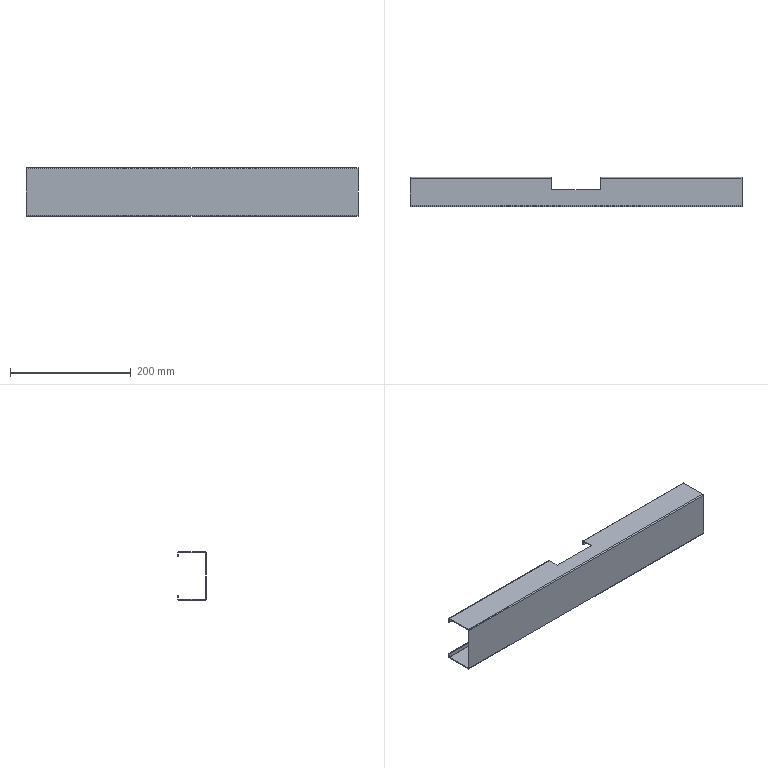Part | 1 solid | 62 faces | box 550 x 48 x 80 mm | volume 145842 mm3 | plane 50 | cylinder 12 | commonest cylinder face diameters 0.4 x6 3.4 x6
STEP:
#1=CARTESIAN_POINT('',(-40.,48.,38.3));
#2=VERTEX_POINT('',#1);
#3=CARTESIAN_POINT('',(-40.,48.,32.));
#4=VERTEX_POINT('',#3);
#5=CARTESIAN_POINT('',(-40.,48.,32.));
#6=DIRECTION('',(0.,0.,-1.));
#7=VECTOR('',#6,1000.);
#8=LINE('',#5,#7);
#9=EDGE_CURVE('',#2,#4,#8,.T.);
#10=ORIENTED_EDGE('',*,*,#9,.F.);
#11=CARTESIAN_POINT('',(-40.,46.5,38.3));
#12=VERTEX_POINT('',#11);
#13=CARTESIAN_POINT('',(-40.,48.,38.3));
#14=DIRECTION('',(0.,-1.,0.));
#15=VECTOR('',#14,1000.);
#16=LINE('',#13,#15);
#17=EDGE_CURVE('',#2,#12,#16,.T.);
#18=ORIENTED_EDGE('',*,*,#17,.T.);
#19=CARTESIAN_POINT('',(-40.,46.5,32.));
#20=VERTEX_POINT('',#19);
#21=CARTESIAN_POINT('',(-40.,46.5,32.));
#22=DIRECTION('',(0.,0.,-1.));
#23=VECTOR('',#22,1000.);
#24=LINE('',#21,#23);
#25=EDGE_CURVE('',#12,#20,#24,.T.);
#26=ORIENTED_EDGE('',*,*,#25,.T.);
#27=CARTESIAN_POINT('',(-40.,48.,32.));
#28=DIRECTION('',(0.,1.,0.));
#29=VECTOR('',#28,1000.);
#30=LINE('',#27,#29);
#31=EDGE_CURVE('',#20,#4,#30,.T.);
#32=ORIENTED_EDGE('',*,*,#31,.T.);
#33=EDGE_LOOP('',(#10,#18,#26,#32));
#34=FACE_OUTER_BOUND('',#33,.T.);
#35=CARTESIAN_POINT('',(-40.,68.,-40.));
#36=DIRECTION('',(-1.,0.,0.));
#37=DIRECTION('',(0.,0.,1.));
#38=AXIS2_PLACEMENT_3D('',#35,#36,#37);
#39=PLANE('',#38);
#40=ADVANCED_FACE('',(#34),#39,.F.);
#41=CARTESIAN_POINT('',(-40.,28.,38.5));
#42=VERTEX_POINT('',#41);
#43=CARTESIAN_POINT('',(-40.,46.3,38.5));
#44=VERTEX_POINT('',#43);
#45=CARTESIAN_POINT('',(-40.,48.,38.5));
#46=DIRECTION('',(0.,1.,0.));
#47=VECTOR('',#46,1000.);
#48=LINE('',#45,#47);
#49=EDGE_CURVE('',#42,#44,#48,.T.);
#50=ORIENTED_EDGE('',*,*,#49,.T.);
#51=CARTESIAN_POINT('',(-40.,46.3,40.));
#52=VERTEX_POINT('',#51);
#53=CARTESIAN_POINT('',(-40.,46.3,38.5));
#54=DIRECTION('',(0.,0.,1.));
#55=VECTOR('',#54,1000.);
#56=LINE('',#53,#55);
#57=EDGE_CURVE('',#44,#52,#56,.T.);
#58=ORIENTED_EDGE('',*,*,#57,.T.);
#59=CARTESIAN_POINT('',(-40.,28.,40.));
#60=VERTEX_POINT('',#59);
#61=CARTESIAN_POINT('',(-40.,48.,40.));
#62=DIRECTION('',(0.,1.,0.));
#63=VECTOR('',#62,1000.);
#64=LINE('',#61,#63);
#65=EDGE_CURVE('',#60,#52,#64,.T.);
#66=ORIENTED_EDGE('',*,*,#65,.F.);
#67=CARTESIAN_POINT('',(-40.,28.,-40.));
#68=DIRECTION('',(0.,0.,1.));
#69=VECTOR('',#68,1000.);
#70=LINE('',#67,#69);
#71=EDGE_CURVE('',#42,#60,#70,.T.);
#72=ORIENTED_EDGE('',*,*,#71,.F.);
#73=EDGE_LOOP('',(#50,#58,#66,#72));
#74=FACE_OUTER_BOUND('',#73,.T.);
#75=CARTESIAN_POINT('',(-40.,68.,-40.));
#76=DIRECTION('',(-1.,0.,0.));
#77=DIRECTION('',(0.,0.,1.));
#78=AXIS2_PLACEMENT_3D('',#75,#76,#77);
#79=PLANE('',#78);
#80=ADVANCED_FACE('',(#74),#79,.F.);
#81=CARTESIAN_POINT('',(40.,46.5,32.));
#82=VERTEX_POINT('',#81);
#83=CARTESIAN_POINT('',(40.,46.5,38.3));
#84=VERTEX_POINT('',#83);
#85=CARTESIAN_POINT('',(40.,46.5,32.));
#86=DIRECTION('',(0.,0.,1.));
#87=VECTOR('',#86,1000.);
#88=LINE('',#85,#87);
#89=EDGE_CURVE('',#82,#84,#88,.T.);
#90=ORIENTED_EDGE('',*,*,#89,.T.);
#91=CARTESIAN_POINT('',(40.,48.,38.3));
#92=VERTEX_POINT('',#91);
#93=CARTESIAN_POINT('',(40.,46.5,38.3));
#94=DIRECTION('',(0.,1.,0.));
#95=VECTOR('',#94,1000.);
#96=LINE('',#93,#95);
#97=EDGE_CURVE('',#84,#92,#96,.T.);
#98=ORIENTED_EDGE('',*,*,#97,.T.);
#99=CARTESIAN_POINT('',(40.,48.,32.));
#100=VERTEX_POINT('',#99);
#101=CARTESIAN_POINT('',(40.,48.,32.));
#102=DIRECTION('',(0.,0.,1.));
#103=VECTOR('',#102,1000.);
#104=LINE('',#101,#103);
#105=EDGE_CURVE('',#100,#92,#104,.T.);
#106=ORIENTED_EDGE('',*,*,#105,.F.);
#107=CARTESIAN_POINT('',(40.,48.,32.));
#108=DIRECTION('',(0.,-1.,0.));
#109=VECTOR('',#108,1000.);
#110=LINE('',#107,#109);
#111=EDGE_CURVE('',#100,#82,#110,.T.);
#112=ORIENTED_EDGE('',*,*,#111,.T.);
#113=EDGE_LOOP('',(#90,#98,#106,#112));
#114=FACE_OUTER_BOUND('',#113,.T.);
#115=CARTESIAN_POINT('',(40.,68.,-40.));
#116=DIRECTION('',(1.,0.,0.));
#117=DIRECTION('',(0.,1.,0.));
#118=AXIS2_PLACEMENT_3D('',#115,#116,#117);
#119=PLANE('',#118);
#120=ADVANCED_FACE('',(#114),#119,.F.);
#121=CARTESIAN_POINT('',(40.,46.3,40.));
#122=VERTEX_POINT('',#121);
#123=CARTESIAN_POINT('',(40.,28.,40.));
#124=VERTEX_POINT('',#123);
#125=CARTESIAN_POINT('',(40.,48.,40.));
#126=DIRECTION('',(0.,-1.,0.));
#127=VECTOR('',#126,1000.);
#128=LINE('',#125,#127);
#129=EDGE_CURVE('',#122,#124,#128,.T.);
#130=ORIENTED_EDGE('',*,*,#129,.F.);
#131=CARTESIAN_POINT('',(40.,46.3,38.5));
#132=VERTEX_POINT('',#131);
#133=CARTESIAN_POINT('',(40.,46.3,40.));
#134=DIRECTION('',(0.,0.,-1.));
#135=VECTOR('',#134,1000.);
#136=LINE('',#133,#135);
#137=EDGE_CURVE('',#122,#132,#136,.T.);
#138=ORIENTED_EDGE('',*,*,#137,.T.);
#139=CARTESIAN_POINT('',(40.,28.,38.5));
#140=VERTEX_POINT('',#139);
#141=CARTESIAN_POINT('',(40.,48.,38.5));
#142=DIRECTION('',(0.,-1.,0.));
#143=VECTOR('',#142,1000.);
#144=LINE('',#141,#143);
#145=EDGE_CURVE('',#132,#140,#144,.T.);
#146=ORIENTED_EDGE('',*,*,#145,.T.);
#147=CARTESIAN_POINT('',(40.,28.,-40.));
#148=DIRECTION('',(0.,0.,1.));
#149=VECTOR('',#148,1000.);
#150=LINE('',#147,#149);
#151=EDGE_CURVE('',#140,#124,#150,.T.);
#152=ORIENTED_EDGE('',*,*,#151,.T.);
#153=EDGE_LOOP('',(#130,#138,#146,#152));
#154=FACE_OUTER_BOUND('',#153,.T.);
#155=CARTESIAN_POINT('',(40.,68.,-40.));
#156=DIRECTION('',(1.,0.,0.));
#157=DIRECTION('',(0.,1.,0.));
#158=AXIS2_PLACEMENT_3D('',#155,#156,#157);
#159=PLANE('',#158);
#160=ADVANCED_FACE('',(#154),#159,.F.);
#161=CARTESIAN_POINT('',(-40.,46.5,-32.));
#162=VERTEX_POINT('',#161);
#163=CARTESIAN_POINT('',(-40.,46.5,-38.3));
#164=VERTEX_POINT('',#163);
#165=CARTESIAN_POINT('',(-40.,46.5,-40.));
#166=DIRECTION('',(0.,0.,-1.));
#167=VECTOR('',#166,1000.);
#168=LINE('',#165,#167);
#169=EDGE_CURVE('',#162,#164,#168,.T.);
#170=ORIENTED_EDGE('',*,*,#169,.T.);
#171=CARTESIAN_POINT('',(-40.,48.,-38.3));
#172=VERTEX_POINT('',#171);
#173=CARTESIAN_POINT('',(-40.,46.5,-38.3));
#174=DIRECTION('',(0.,1.,0.));
#175=VECTOR('',#174,1000.);
#176=LINE('',#173,#175);
#177=EDGE_CURVE('',#164,#172,#176,.T.);
#178=ORIENTED_EDGE('',*,*,#177,.T.);
#179=CARTESIAN_POINT('',(-40.,48.,-32.));
#180=VERTEX_POINT('',#179);
#181=CARTESIAN_POINT('',(-40.,48.,-40.));
#182=DIRECTION('',(0.,0.,-1.));
#183=VECTOR('',#182,1000.);
#184=LINE('',#181,#183);
#185=EDGE_CURVE('',#180,#172,#184,.T.);
#186=ORIENTED_EDGE('',*,*,#185,.F.);
#187=CARTESIAN_POINT('',(-40.,46.5,-32.));
#188=DIRECTION('',(0.,-1.,0.));
#189=VECTOR('',#188,1000.);
#190=LINE('',#187,#189);
#191=EDGE_CURVE('',#180,#162,#190,.T.);
#192=ORIENTED_EDGE('',*,*,#191,.T.);
#193=EDGE_LOOP('',(#170,#178,#186,#192));
#194=FACE_OUTER_BOUND('',#193,.T.);
#195=CARTESIAN_POINT('',(-40.,68.,-40.));
#196=DIRECTION('',(-1.,0.,0.));
#197=DIRECTION('',(0.,0.,1.));
#198=AXIS2_PLACEMENT_3D('',#195,#196,#197);
#199=PLANE('',#198);
#200=ADVANCED_FACE('',(#194),#199,.F.);
#201=CARTESIAN_POINT('',(-40.,46.3,-40.));
#202=VERTEX_POINT('',#201);
#203=CARTESIAN_POINT('',(-40.,28.,-40.));
#204=VERTEX_POINT('',#203);
#205=CARTESIAN_POINT('',(-40.,68.,-40.));
#206=DIRECTION('',(0.,-1.,0.));
#207=VECTOR('',#206,1000.);
#208=LINE('',#205,#207);
#209=EDGE_CURVE('',#202,#204,#208,.T.);
#210=ORIENTED_EDGE('',*,*,#209,.F.);
#211=CARTESIAN_POINT('',(-40.,46.3,-38.5));
#212=VERTEX_POINT('',#211);
#213=CARTESIAN_POINT('',(-40.,46.3,-40.));
#214=DIRECTION('',(0.,0.,1.));
#215=VECTOR('',#214,1000.);
#216=LINE('',#213,#215);
#217=EDGE_CURVE('',#202,#212,#216,.T.);
#218=ORIENTED_EDGE('',*,*,#217,.T.);
#219=CARTESIAN_POINT('',(-40.,28.,-38.5));
#220=VERTEX_POINT('',#219);
#221=CARTESIAN_POINT('',(-40.,0.,-38.5));
#222=DIRECTION('',(0.,-1.,0.));
#223=VECTOR('',#222,1000.);
#224=LINE('',#221,#223);
#225=EDGE_CURVE('',#212,#220,#224,.T.);
#226=ORIENTED_EDGE('',*,*,#225,.T.);
#227=CARTESIAN_POINT('',(-40.,28.,-40.));
#228=DIRECTION('',(0.,0.,1.));
#229=VECTOR('',#228,1000.);
#230=LINE('',#227,#229);
#231=EDGE_CURVE('',#204,#220,#230,.T.);
#232=ORIENTED_EDGE('',*,*,#231,.F.);
#233=EDGE_LOOP('',(#210,#218,#226,#232));
#234=FACE_OUTER_BOUND('',#233,.T.);
#235=CARTESIAN_POINT('',(-40.,68.,-40.));
#236=DIRECTION('',(-1.,0.,0.));
#237=DIRECTION('',(0.,0.,1.));
#238=AXIS2_PLACEMENT_3D('',#235,#236,#237);
#239=PLANE('',#238);
#240=ADVANCED_FACE('',(#234),#239,.F.);
#241=CARTESIAN_POINT('',(40.,48.,-38.3));
#242=VERTEX_POINT('',#241);
#243=CARTESIAN_POINT('',(40.,48.,-32.));
#244=VERTEX_POINT('',#243);
#245=CARTESIAN_POINT('',(40.,48.,-40.));
#246=DIRECTION('',(0.,0.,1.));
#247=VECTOR('',#246,1000.);
#248=LINE('',#245,#247);
#249=EDGE_CURVE('',#242,#244,#248,.T.);
#250=ORIENTED_EDGE('',*,*,#249,.F.);
#251=CARTESIAN_POINT('',(40.,46.5,-38.3));
#252=VERTEX_POINT('',#251);
#253=CARTESIAN_POINT('',(40.,48.,-38.3));
#254=DIRECTION('',(0.,-1.,0.));
#255=VECTOR('',#254,1000.);
#256=LINE('',#253,#255);
#257=EDGE_CURVE('',#242,#252,#256,.T.);
#258=ORIENTED_EDGE('',*,*,#257,.T.);
#259=CARTESIAN_POINT('',(40.,46.5,-32.));
#260=VERTEX_POINT('',#259);
#261=CARTESIAN_POINT('',(40.,46.5,-40.));
#262=DIRECTION('',(0.,0.,1.));
#263=VECTOR('',#262,1000.);
#264=LINE('',#261,#263);
#265=EDGE_CURVE('',#252,#260,#264,.T.);
#266=ORIENTED_EDGE('',*,*,#265,.T.);
#267=CARTESIAN_POINT('',(40.,46.5,-32.));
#268=DIRECTION('',(0.,1.,0.));
#269=VECTOR('',#268,1000.);
#270=LINE('',#267,#269);
#271=EDGE_CURVE('',#260,#244,#270,.T.);
#272=ORIENTED_EDGE('',*,*,#271,.T.);
#273=EDGE_LOOP('',(#250,#258,#266,#272));
#274=FACE_OUTER_BOUND('',#273,.T.);
#275=CARTESIAN_POINT('',(40.,68.,-40.));
#276=DIRECTION('',(1.,0.,0.));
#277=DIRECTION('',(0.,1.,0.));
#278=AXIS2_PLACEMENT_3D('',#275,#276,#277);
#279=PLANE('',#278);
#280=ADVANCED_FACE('',(#274),#279,.F.);
#281=CARTESIAN_POINT('',(40.,28.,-38.5));
#282=VERTEX_POINT('',#281);
#283=CARTESIAN_POINT('',(40.,46.3,-38.5));
#284=VERTEX_POINT('',#283);
#285=CARTESIAN_POINT('',(40.,0.,-38.5));
#286=DIRECTION('',(0.,1.,0.));
#287=VECTOR('',#286,1000.);
#288=LINE('',#285,#287);
#289=EDGE_CURVE('',#282,#284,#288,.T.);
#290=ORIENTED_EDGE('',*,*,#289,.T.);
#291=CARTESIAN_POINT('',(40.,46.3,-40.));
#292=VERTEX_POINT('',#291);
#293=CARTESIAN_POINT('',(40.,46.3,-38.5));
#294=DIRECTION('',(0.,0.,-1.));
#295=VECTOR('',#294,1000.);
#296=LINE('',#293,#295);
#297=EDGE_CURVE('',#284,#292,#296,.T.);
#298=ORIENTED_EDGE('',*,*,#297,.T.);
#299=CARTESIAN_POINT('',(40.,28.,-40.));
#300=VERTEX_POINT('',#299);
#301=CARTESIAN_POINT('',(40.,68.,-40.));
#302=DIRECTION('',(0.,1.,0.));
#303=VECTOR('',#302,1000.);
#304=LINE('',#301,#303);
#305=EDGE_CURVE('',#300,#292,#304,.T.);
#306=ORIENTED_EDGE('',*,*,#305,.F.);
#307=CARTESIAN_POINT('',(40.,28.,-40.));
#308=DIRECTION('',(0.,0.,1.));
#309=VECTOR('',#308,1000.);
#310=LINE('',#307,#309);
#311=EDGE_CURVE('',#300,#282,#310,.T.);
#312=ORIENTED_EDGE('',*,*,#311,.T.);
#313=EDGE_LOOP('',(#290,#298,#306,#312));
#314=FACE_OUTER_BOUND('',#313,.T.);
#315=CARTESIAN_POINT('',(40.,68.,-40.));
#316=DIRECTION('',(1.,0.,0.));
#317=DIRECTION('',(0.,1.,0.));
#318=AXIS2_PLACEMENT_3D('',#315,#316,#317);
#319=PLANE('',#318);
#320=ADVANCED_FACE('',(#314),#319,.F.);
#321=CARTESIAN_POINT('',(275.,48.,-38.3));
#322=VERTEX_POINT('',#321);
#323=CARTESIAN_POINT('',(275.,48.,-38.3));
#324=DIRECTION('',(-1.,0.,0.));
#325=VECTOR('',#324,1000.);
#326=LINE('',#323,#325);
#327=EDGE_CURVE('',#322,#242,#326,.T.);
#328=ORIENTED_EDGE('',*,*,#327,.T.);
#329=ORIENTED_EDGE('',*,*,#249,.T.);
#330=CARTESIAN_POINT('',(275.,48.,-32.));
#331=VERTEX_POINT('',#330);
#332=CARTESIAN_POINT('',(275.,48.,-32.));
#333=DIRECTION('',(-1.,0.,0.));
#334=VECTOR('',#333,1000.);
#335=LINE('',#332,#334);
#336=EDGE_CURVE('',#331,#244,#335,.T.);
#337=ORIENTED_EDGE('',*,*,#336,.F.);
#338=CARTESIAN_POINT('',(275.,48.,-40.));
#339=DIRECTION('',(0.,0.,1.));
#340=VECTOR('',#339,1000.);
#341=LINE('',#338,#340);
#342=EDGE_CURVE('',#322,#331,#341,.T.);
#343=ORIENTED_EDGE('',*,*,#342,.F.);
#344=EDGE_LOOP('',(#328,#329,#337,#343));
#345=FACE_OUTER_BOUND('',#344,.T.);
#346=CARTESIAN_POINT('',(275.,48.,-40.));
#347=DIRECTION('',(0.,-1.,0.));
#348=DIRECTION('',(0.,0.,-1.));
#349=AXIS2_PLACEMENT_3D('',#346,#347,#348);
#350=PLANE('',#349);
#351=ADVANCED_FACE('',(#345),#350,.F.);
#352=ORIENTED_EDGE('',*,*,#271,.F.);
#353=CARTESIAN_POINT('',(275.,46.5,-32.));
#354=VERTEX_POINT('',#353);
#355=CARTESIAN_POINT('',(275.,46.5,-32.));
#356=DIRECTION('',(-1.,0.,0.));
#357=VECTOR('',#356,1000.);
#358=LINE('',#355,#357);
#359=EDGE_CURVE('',#354,#260,#358,.T.);
#360=ORIENTED_EDGE('',*,*,#359,.F.);
#361=CARTESIAN_POINT('',(275.,46.5,-32.));
#362=DIRECTION('',(0.,1.,0.));
#363=VECTOR('',#362,1000.);
#364=LINE('',#361,#363);
#365=EDGE_CURVE('',#354,#331,#364,.T.);
#366=ORIENTED_EDGE('',*,*,#365,.T.);
#367=ORIENTED_EDGE('',*,*,#336,.T.);
#368=EDGE_LOOP('',(#352,#360,#366,#367));
#369=FACE_OUTER_BOUND('',#368,.T.);
#370=CARTESIAN_POINT('',(275.,46.5,-32.));
#371=DIRECTION('',(0.,0.,1.));
#372=DIRECTION('',(1.,0.,0.));
#373=AXIS2_PLACEMENT_3D('',#370,#371,#372);
#374=PLANE('',#373);
#375=ADVANCED_FACE('',(#369),#374,.T.);
#376=ORIENTED_EDGE('',*,*,#265,.F.);
#377=CARTESIAN_POINT('',(275.,46.5,-38.3));
#378=VERTEX_POINT('',#377);
#379=CARTESIAN_POINT('',(275.,46.5,-38.3));
#380=DIRECTION('',(-1.,0.,0.));
#381=VECTOR('',#380,1000.);
#382=LINE('',#379,#381);
#383=EDGE_CURVE('',#378,#252,#382,.T.);
#384=ORIENTED_EDGE('',*,*,#383,.F.);
#385=CARTESIAN_POINT('',(275.,46.5,-40.));
#386=DIRECTION('',(0.,0.,1.));
#387=VECTOR('',#386,1000.);
#388=LINE('',#385,#387);
#389=EDGE_CURVE('',#378,#354,#388,.T.);
#390=ORIENTED_EDGE('',*,*,#389,.T.);
#391=ORIENTED_EDGE('',*,*,#359,.T.);
#392=EDGE_LOOP('',(#376,#384,#390,#391));
#393=FACE_OUTER_BOUND('',#392,.T.);
#394=CARTESIAN_POINT('',(275.,46.5,-40.));
#395=DIRECTION('',(0.,-1.,0.));
#396=DIRECTION('',(0.,0.,-1.));
#397=AXIS2_PLACEMENT_3D('',#394,#395,#396);
#398=PLANE('',#397);
#399=ADVANCED_FACE('',(#393),#398,.T.);
#400=CARTESIAN_POINT('',(40.,46.3,-38.3));
#401=DIRECTION('',(1.,0.,0.));
#402=DIRECTION('',(0.,1.,0.));
#403=AXIS2_PLACEMENT_3D('',#400,#401,#402);
#404=CIRCLE('',#403,0.2);
#405=EDGE_CURVE('',#284,#252,#404,.T.);
#406=ORIENTED_EDGE('',*,*,#405,.F.);
#407=CARTESIAN_POINT('',(275.,46.3,-38.5));
#408=VERTEX_POINT('',#407);
#409=CARTESIAN_POINT('',(275.,46.3,-38.5));
#410=DIRECTION('',(-1.,0.,0.));
#411=VECTOR('',#410,1000.);
#412=LINE('',#409,#411);
#413=EDGE_CURVE('',#408,#284,#412,.T.);
#414=ORIENTED_EDGE('',*,*,#413,.F.);
#415=CARTESIAN_POINT('',(275.,46.3,-38.3));
#416=DIRECTION('',(1.,0.,0.));
#417=DIRECTION('',(0.,0.,-1.));
#418=AXIS2_PLACEMENT_3D('',#415,#416,#417);
#419=CIRCLE('',#418,0.2);
#420=EDGE_CURVE('',#408,#378,#419,.T.);
#421=ORIENTED_EDGE('',*,*,#420,.T.);
#422=ORIENTED_EDGE('',*,*,#383,.T.);
#423=EDGE_LOOP('',(#406,#414,#421,#422));
#424=FACE_OUTER_BOUND('',#423,.T.);
#425=CARTESIAN_POINT('',(275.,46.3,-38.3));
#426=DIRECTION('',(-1.,0.,0.));
#427=DIRECTION('',(0.,0.,1.));
#428=AXIS2_PLACEMENT_3D('',#425,#426,#427);
#429=CYLINDRICAL_SURFACE('',#428,0.2);
#430=ADVANCED_FACE('',(#424),#429,.F.);
#431=CARTESIAN_POINT('',(40.,46.3,38.3));
#432=DIRECTION('',(1.,0.,0.));
#433=DIRECTION('',(0.,1.,0.));
#434=AXIS2_PLACEMENT_3D('',#431,#432,#433);
#435=CIRCLE('',#434,0.2);
#436=EDGE_CURVE('',#84,#132,#435,.T.);
#437=ORIENTED_EDGE('',*,*,#436,.F.);
#438=CARTESIAN_POINT('',(275.,46.5,38.3));
#439=VERTEX_POINT('',#438);
#440=CARTESIAN_POINT('',(275.,46.5,38.3));
#441=DIRECTION('',(-1.,0.,0.));
#442=VECTOR('',#441,1000.);
#443=LINE('',#440,#442);
#444=EDGE_CURVE('',#439,#84,#443,.T.);
#445=ORIENTED_EDGE('',*,*,#444,.F.);
#446=CARTESIAN_POINT('',(275.,46.3,38.5));
#447=VERTEX_POINT('',#446);
#448=CARTESIAN_POINT('',(275.,46.3,38.3));
#449=DIRECTION('',(1.,0.,0.));
#450=DIRECTION('',(0.,0.,-1.));
#451=AXIS2_PLACEMENT_3D('',#448,#449,#450);
#452=CIRCLE('',#451,0.2);
#453=EDGE_CURVE('',#439,#447,#452,.T.);
#454=ORIENTED_EDGE('',*,*,#453,.T.);
#455=CARTESIAN_POINT('',(275.,46.3,38.5));
#456=DIRECTION('',(-1.,0.,0.));
#457=VECTOR('',#456,1000.);
#458=LINE('',#455,#457);
#459=EDGE_CURVE('',#447,#132,#458,.T.);
#460=ORIENTED_EDGE('',*,*,#459,.T.);
#461=EDGE_LOOP('',(#437,#445,#454,#460));
#462=FACE_OUTER_BOUND('',#461,.T.);
#463=CARTESIAN_POINT('',(275.,46.3,38.3));
#464=DIRECTION('',(-1.,0.,0.));
#465=DIRECTION('',(0.,0.,1.));
#466=AXIS2_PLACEMENT_3D('',#463,#464,#465);
#467=CYLINDRICAL_SURFACE('',#466,0.2);
#468=ADVANCED_FACE('',(#462),#467,.F.);
#469=ORIENTED_EDGE('',*,*,#89,.F.);
#470=CARTESIAN_POINT('',(275.,46.5,32.));
#471=VERTEX_POINT('',#470);
#472=CARTESIAN_POINT('',(275.,46.5,32.));
#473=DIRECTION('',(-1.,0.,0.));
#474=VECTOR('',#473,1000.);
#475=LINE('',#472,#474);
#476=EDGE_CURVE('',#471,#82,#475,.T.);
#477=ORIENTED_EDGE('',*,*,#476,.F.);
#478=CARTESIAN_POINT('',(275.,46.5,32.));
#479=DIRECTION('',(0.,0.,1.));
#480=VECTOR('',#479,1000.);
#481=LINE('',#478,#480);
#482=EDGE_CURVE('',#471,#439,#481,.T.);
#483=ORIENTED_EDGE('',*,*,#482,.T.);
#484=ORIENTED_EDGE('',*,*,#444,.T.);
#485=EDGE_LOOP('',(#469,#477,#483,#484));
#486=FACE_OUTER_BOUND('',#485,.T.);
#487=CARTESIAN_POINT('',(275.,46.5,32.));
#488=DIRECTION('',(0.,-1.,0.));
#489=DIRECTION('',(0.,0.,-1.));
#490=AXIS2_PLACEMENT_3D('',#487,#488,#489);
#491=PLANE('',#490);
#492=ADVANCED_FACE('',(#486),#491,.T.);
#493=ORIENTED_EDGE('',*,*,#111,.F.);
#494=CARTESIAN_POINT('',(275.,48.,32.));
#495=VERTEX_POINT('',#494);
#496=CARTESIAN_POINT('',(275.,48.,32.));
#497=DIRECTION('',(-1.,0.,0.));
#498=VECTOR('',#497,1000.);
#499=LINE('',#496,#498);
#500=EDGE_CURVE('',#495,#100,#499,.T.);
#501=ORIENTED_EDGE('',*,*,#500,.F.);
#502=CARTESIAN_POINT('',(275.,48.,32.));
#503=DIRECTION('',(0.,-1.,0.));
#504=VECTOR('',#503,1000.);
#505=LINE('',#502,#504);
#506=EDGE_CURVE('',#495,#471,#505,.T.);
#507=ORIENTED_EDGE('',*,*,#506,.T.);
#508=ORIENTED_EDGE('',*,*,#476,.T.);
#509=EDGE_LOOP('',(#493,#501,#507,#508));
#510=FACE_OUTER_BOUND('',#509,.T.);
#511=CARTESIAN_POINT('',(275.,48.,32.));
#512=DIRECTION('',(0.,0.,-1.));
#513=DIRECTION('',(-1.,0.,0.));
#514=AXIS2_PLACEMENT_3D('',#511,#512,#513);
#515=PLANE('',#514);
#516=ADVANCED_FACE('',(#510),#515,.T.);
#517=ORIENTED_EDGE('',*,*,#500,.T.);
#518=ORIENTED_EDGE('',*,*,#105,.T.);
#519=CARTESIAN_POINT('',(275.,48.,38.3));
#520=VERTEX_POINT('',#519);
#521=CARTESIAN_POINT('',(275.,48.,38.3));
#522=DIRECTION('',(-1.,0.,0.));
#523=VECTOR('',#522,1000.);
#524=LINE('',#521,#523);
#525=EDGE_CURVE('',#520,#92,#524,.T.);
#526=ORIENTED_EDGE('',*,*,#525,.F.);
#527=CARTESIAN_POINT('',(275.,48.,32.));
#528=DIRECTION('',(0.,0.,1.));
#529=VECTOR('',#528,1000.);
#530=LINE('',#527,#529);
#531=EDGE_CURVE('',#495,#520,#530,.T.);
#532=ORIENTED_EDGE('',*,*,#531,.F.);
#533=EDGE_LOOP('',(#517,#518,#526,#532));
#534=FACE_OUTER_BOUND('',#533,.T.);
#535=CARTESIAN_POINT('',(275.,48.,32.));
#536=DIRECTION('',(0.,-1.,0.));
#537=DIRECTION('',(0.,0.,-1.));
#538=AXIS2_PLACEMENT_3D('',#535,#536,#537);
#539=PLANE('',#538);
#540=ADVANCED_FACE('',(#534),#539,.F.);
#541=ORIENTED_EDGE('',*,*,#525,.T.);
#542=CARTESIAN_POINT('',(40.,46.3,38.3));
#543=DIRECTION('',(1.,0.,0.));
#544=DIRECTION('',(0.,1.,0.));
#545=AXIS2_PLACEMENT_3D('',#542,#543,#544);
#546=CIRCLE('',#545,1.7);
#547=EDGE_CURVE('',#92,#122,#546,.T.);
#548=ORIENTED_EDGE('',*,*,#547,.T.);
#549=CARTESIAN_POINT('',(275.,46.3,40.));
#550=VERTEX_POINT('',#549);
#551=CARTESIAN_POINT('',(275.,46.3,40.));
#552=DIRECTION('',(-1.,0.,0.));
#553=VECTOR('',#552,1000.);
#554=LINE('',#551,#553);
#555=EDGE_CURVE('',#550,#122,#554,.T.);
#556=ORIENTED_EDGE('',*,*,#555,.F.);
#557=CARTESIAN_POINT('',(275.,46.3,38.3));
#558=DIRECTION('',(1.,0.,0.));
#559=DIRECTION('',(0.,0.,1.));
#560=AXIS2_PLACEMENT_3D('',#557,#558,#559);
#561=CIRCLE('',#560,1.7);
#562=EDGE_CURVE('',#520,#550,#561,.T.);
#563=ORIENTED_EDGE('',*,*,#562,.F.);
#564=EDGE_LOOP('',(#541,#548,#556,#563));
#565=FACE_OUTER_BOUND('',#564,.T.);
#566=CARTESIAN_POINT('',(275.,46.3,38.3));
#567=DIRECTION('',(-1.,0.,0.));
#568=DIRECTION('',(0.,0.,1.));
#569=AXIS2_PLACEMENT_3D('',#566,#567,#568);
#570=CYLINDRICAL_SURFACE('',#569,1.7);
#571=ADVANCED_FACE('',(#565),#570,.T.);
#572=CARTESIAN_POINT('',(275.,46.3,-40.));
#573=VERTEX_POINT('',#572);
#574=CARTESIAN_POINT('',(275.,46.3,-40.));
#575=DIRECTION('',(-1.,0.,0.));
#576=VECTOR('',#575,1000.);
#577=LINE('',#574,#576);
#578=EDGE_CURVE('',#573,#292,#577,.T.);
#579=ORIENTED_EDGE('',*,*,#578,.T.);
#580=CARTESIAN_POINT('',(40.,46.3,-38.3));
#581=DIRECTION('',(1.,0.,0.));
#582=DIRECTION('',(0.,1.,0.));
#583=AXIS2_PLACEMENT_3D('',#580,#581,#582);
#584=CIRCLE('',#583,1.7);
#585=EDGE_CURVE('',#292,#242,#584,.T.);
#586=ORIENTED_EDGE('',*,*,#585,.T.);
#587=ORIENTED_EDGE('',*,*,#327,.F.);
#588=CARTESIAN_POINT('',(275.,46.3,-38.3));
#589=DIRECTION('',(1.,0.,0.));
#590=DIRECTION('',(0.,0.,1.));
#591=AXIS2_PLACEMENT_3D('',#588,#589,#590);
#592=CIRCLE('',#591,1.7);
#593=EDGE_CURVE('',#573,#322,#592,.T.);
#594=ORIENTED_EDGE('',*,*,#593,.F.);
#595=EDGE_LOOP('',(#579,#586,#587,#594));
#596=FACE_OUTER_BOUND('',#595,.T.);
#597=CARTESIAN_POINT('',(275.,46.3,-38.3));
#598=DIRECTION('',(-1.,0.,0.));
#599=DIRECTION('',(0.,0.,1.));
#600=AXIS2_PLACEMENT_3D('',#597,#598,#599);
#601=CYLINDRICAL_SURFACE('',#600,1.7);
#602=ADVANCED_FACE('',(#596),#601,.T.);
#603=CARTESIAN_POINT('',(275.,48.,38.3));
#604=DIRECTION('',(0.,-1.,0.));
#605=VECTOR('',#604,1000.);
#606=LINE('',#603,#605);
#607=EDGE_CURVE('',#520,#439,#606,.T.);
#608=ORIENTED_EDGE('',*,*,#607,.F.);
#609=ORIENTED_EDGE('',*,*,#562,.T.);
#610=CARTESIAN_POINT('',(275.,46.3,38.5));
#611=DIRECTION('',(0.,0.,1.));
#612=VECTOR('',#611,1000.);
#613=LINE('',#610,#612);
#614=EDGE_CURVE('',#447,#550,#613,.T.);
#615=ORIENTED_EDGE('',*,*,#614,.F.);
#616=ORIENTED_EDGE('',*,*,#453,.F.);
#617=EDGE_LOOP('',(#608,#609,#615,#616));
#618=FACE_OUTER_BOUND('',#617,.T.);
#619=CARTESIAN_POINT('',(275.,48.,38.3));
#620=DIRECTION('',(1.,0.,0.));
#621=DIRECTION('',(0.,0.,-1.));
#622=AXIS2_PLACEMENT_3D('',#619,#620,#621);
#623=PLANE('',#622);
#624=ADVANCED_FACE('',(#618),#623,.T.);
#625=ORIENTED_EDGE('',*,*,#531,.T.);
#626=ORIENTED_EDGE('',*,*,#607,.T.);
#627=ORIENTED_EDGE('',*,*,#482,.F.);
#628=ORIENTED_EDGE('',*,*,#506,.F.);
#629=EDGE_LOOP('',(#625,#626,#627,#628));
#630=FACE_OUTER_BOUND('',#629,.T.);
#631=CARTESIAN_POINT('',(275.,46.3,38.5));
#632=DIRECTION('',(1.,0.,0.));
#633=DIRECTION('',(0.,0.,-1.));
#634=AXIS2_PLACEMENT_3D('',#631,#632,#633);
#635=PLANE('',#634);
#636=ADVANCED_FACE('',(#630),#635,.T.);
#637=CARTESIAN_POINT('',(-275.,46.3,40.));
#638=VERTEX_POINT('',#637);
#639=CARTESIAN_POINT('',(-275.,46.3,38.5));
#640=VERTEX_POINT('',#639);
#641=CARTESIAN_POINT('',(-275.,46.3,40.));
#642=DIRECTION('',(0.,0.,-1.));
#643=VECTOR('',#642,1000.);
#644=LINE('',#641,#643);
#645=EDGE_CURVE('',#638,#640,#644,.T.);
#646=ORIENTED_EDGE('',*,*,#645,.F.);
#647=CARTESIAN_POINT('',(-275.,48.,38.3));
#648=VERTEX_POINT('',#647);
#649=CARTESIAN_POINT('',(-275.,46.3,38.3));
#650=DIRECTION('',(1.,0.,0.));
#651=DIRECTION('',(0.,0.,1.));
#652=AXIS2_PLACEMENT_3D('',#649,#650,#651);
#653=CIRCLE('',#652,1.7);
#654=EDGE_CURVE('',#648,#638,#653,.T.);
#655=ORIENTED_EDGE('',*,*,#654,.F.);
#656=CARTESIAN_POINT('',(-275.,46.5,38.3));
#657=VERTEX_POINT('',#656);
#658=CARTESIAN_POINT('',(-275.,46.5,38.3));
#659=DIRECTION('',(0.,1.,0.));
#660=VECTOR('',#659,1000.);
#661=LINE('',#658,#660);
#662=EDGE_CURVE('',#657,#648,#661,.T.);
#663=ORIENTED_EDGE('',*,*,#662,.F.);
#664=CARTESIAN_POINT('',(-275.,46.3,38.3));
#665=DIRECTION('',(1.,0.,0.));
#666=DIRECTION('',(0.,0.,-1.));
#667=AXIS2_PLACEMENT_3D('',#664,#665,#666);
#668=CIRCLE('',#667,0.2);
#669=EDGE_CURVE('',#657,#640,#668,.T.);
#670=ORIENTED_EDGE('',*,*,#669,.T.);
#671=EDGE_LOOP('',(#646,#655,#663,#670));
#672=FACE_OUTER_BOUND('',#671,.T.);
#673=CARTESIAN_POINT('',(-275.,46.3,40.));
#674=DIRECTION('',(-1.,0.,0.));
#675=DIRECTION('',(0.,0.,1.));
#676=AXIS2_PLACEMENT_3D('',#673,#674,#675);
#677=PLANE('',#676);
#678=ADVANCED_FACE('',(#672),#677,.T.);
#679=CARTESIAN_POINT('',(-275.,1.7,40.));
#680=VERTEX_POINT('',#679);
#681=CARTESIAN_POINT('',(-275.,48.,40.));
#682=DIRECTION('',(0.,-1.,0.));
#683=VECTOR('',#682,1000.);
#684=LINE('',#681,#683);
#685=EDGE_CURVE('',#638,#680,#684,.T.);
#686=ORIENTED_EDGE('',*,*,#685,.F.);
#687=ORIENTED_EDGE('',*,*,#645,.T.);
#688=CARTESIAN_POINT('',(-275.,1.7,38.5));
#689=VERTEX_POINT('',#688);
#690=CARTESIAN_POINT('',(-275.,48.,38.5));
#691=DIRECTION('',(0.,-1.,0.));
#692=VECTOR('',#691,1000.);
#693=LINE('',#690,#692);
#694=EDGE_CURVE('',#640,#689,#693,.T.);
#695=ORIENTED_EDGE('',*,*,#694,.T.);
#696=CARTESIAN_POINT('',(-275.,1.7,38.5));
#697=DIRECTION('',(0.,0.,1.));
#698=VECTOR('',#697,1000.);
#699=LINE('',#696,#698);
#700=EDGE_CURVE('',#689,#680,#699,.T.);
#701=ORIENTED_EDGE('',*,*,#700,.T.);
#702=EDGE_LOOP('',(#686,#687,#695,#701));
#703=FACE_OUTER_BOUND('',#702,.T.);
#704=CARTESIAN_POINT('',(-275.,46.5,38.3));
#705=DIRECTION('',(-1.,0.,0.));
#706=DIRECTION('',(0.,0.,1.));
#707=AXIS2_PLACEMENT_3D('',#704,#705,#706);
#708=PLANE('',#707);
#709=ADVANCED_FACE('',(#703),#708,.T.);
#710=CARTESIAN_POINT('',(275.,1.7,40.));
#711=VERTEX_POINT('',#710);
#712=CARTESIAN_POINT('',(275.,1.7,38.5));
#713=VERTEX_POINT('',#712);
#714=CARTESIAN_POINT('',(275.,1.7,40.));
#715=DIRECTION('',(0.,0.,-1.));
#716=VECTOR('',#715,1000.);
#717=LINE('',#714,#716);
#718=EDGE_CURVE('',#711,#713,#717,.T.);
#719=ORIENTED_EDGE('',*,*,#718,.F.);
#720=CARTESIAN_POINT('',(275.,0.,38.3));
#721=VERTEX_POINT('',#720);
#722=CARTESIAN_POINT('',(275.,1.7,38.3));
#723=DIRECTION('',(1.,0.,0.));
#724=DIRECTION('',(0.,0.,1.));
#725=AXIS2_PLACEMENT_3D('',#722,#723,#724);
#726=CIRCLE('',#725,1.7);
#727=EDGE_CURVE('',#711,#721,#726,.T.);
#728=ORIENTED_EDGE('',*,*,#727,.T.);
#729=CARTESIAN_POINT('',(275.,1.5,38.3));
#730=VERTEX_POINT('',#729);
#731=CARTESIAN_POINT('',(275.,1.5,38.3));
#732=DIRECTION('',(0.,-1.,0.));
#733=VECTOR('',#732,1000.);
#734=LINE('',#731,#733);
#735=EDGE_CURVE('',#730,#721,#734,.T.);
#736=ORIENTED_EDGE('',*,*,#735,.F.);
#737=CARTESIAN_POINT('',(275.,1.7,38.3));
#738=DIRECTION('',(1.,0.,0.));
#739=DIRECTION('',(0.,0.,-1.));
#740=AXIS2_PLACEMENT_3D('',#737,#738,#739);
#741=CIRCLE('',#740,0.2);
#742=EDGE_CURVE('',#713,#730,#741,.T.);
#743=ORIENTED_EDGE('',*,*,#742,.F.);
#744=EDGE_LOOP('',(#719,#728,#736,#743));
#745=FACE_OUTER_BOUND('',#744,.T.);
#746=CARTESIAN_POINT('',(275.,1.7,40.));
#747=DIRECTION('',(1.,0.,0.));
#748=DIRECTION('',(0.,0.,-1.));
#749=AXIS2_PLACEMENT_3D('',#746,#747,#748);
#750=PLANE('',#749);
#751=ADVANCED_FACE('',(#745),#750,.T.);
#752=CARTESIAN_POINT('',(275.,48.,40.));
#753=DIRECTION('',(0.,-1.,0.));
#754=VECTOR('',#753,1000.);
#755=LINE('',#752,#754);
#756=EDGE_CURVE('',#550,#711,#755,.T.);
#757=ORIENTED_EDGE('',*,*,#756,.T.);
#758=ORIENTED_EDGE('',*,*,#718,.T.);
#759=CARTESIAN_POINT('',(275.,48.,38.5));
#760=DIRECTION('',(0.,-1.,0.));
#761=VECTOR('',#760,1000.);
#762=LINE('',#759,#761);
#763=EDGE_CURVE('',#447,#713,#762,.T.);
#764=ORIENTED_EDGE('',*,*,#763,.F.);
#765=ORIENTED_EDGE('',*,*,#614,.T.);
#766=EDGE_LOOP('',(#757,#758,#764,#765));
#767=FACE_OUTER_BOUND('',#766,.T.);
#768=CARTESIAN_POINT('',(275.,1.5,38.3));
#769=DIRECTION('',(1.,0.,0.));
#770=DIRECTION('',(0.,0.,-1.));
#771=AXIS2_PLACEMENT_3D('',#768,#769,#770);
#772=PLANE('',#771);
#773=ADVANCED_FACE('',(#767),#772,.T.);
#774=CARTESIAN_POINT('',(-275.,0.,38.3));
#775=VERTEX_POINT('',#774);
#776=CARTESIAN_POINT('',(-275.,1.5,38.3));
#777=VERTEX_POINT('',#776);
#778=CARTESIAN_POINT('',(-275.,0.,38.3));
#779=DIRECTION('',(0.,1.,0.));
#780=VECTOR('',#779,1000.);
#781=LINE('',#778,#780);
#782=EDGE_CURVE('',#775,#777,#781,.T.);
#783=ORIENTED_EDGE('',*,*,#782,.F.);
#784=CARTESIAN_POINT('',(-275.,1.7,38.3));
#785=DIRECTION('',(1.,0.,0.));
#786=DIRECTION('',(0.,0.,1.));
#787=AXIS2_PLACEMENT_3D('',#784,#785,#786);
#788=CIRCLE('',#787,1.7);
#789=EDGE_CURVE('',#680,#775,#788,.T.);
#790=ORIENTED_EDGE('',*,*,#789,.F.);
#791=ORIENTED_EDGE('',*,*,#700,.F.);
#792=CARTESIAN_POINT('',(-275.,1.7,38.3));
#793=DIRECTION('',(1.,0.,0.));
#794=DIRECTION('',(0.,0.,-1.));
#795=AXIS2_PLACEMENT_3D('',#792,#793,#794);
#796=CIRCLE('',#795,0.2);
#797=EDGE_CURVE('',#689,#777,#796,.T.);
#798=ORIENTED_EDGE('',*,*,#797,.T.);
#799=EDGE_LOOP('',(#783,#790,#791,#798));
#800=FACE_OUTER_BOUND('',#799,.T.);
#801=CARTESIAN_POINT('',(-275.,0.,38.3));
#802=DIRECTION('',(-1.,0.,0.));
#803=DIRECTION('',(0.,0.,1.));
#804=AXIS2_PLACEMENT_3D('',#801,#802,#803);
#805=PLANE('',#804);
#806=ADVANCED_FACE('',(#800),#805,.T.);
#807=CARTESIAN_POINT('',(-275.,0.,-38.3));
#808=VERTEX_POINT('',#807);
#809=CARTESIAN_POINT('',(-275.,0.,40.));
#810=DIRECTION('',(0.,0.,-1.));
#811=VECTOR('',#810,1000.);
#812=LINE('',#809,#811);
#813=EDGE_CURVE('',#775,#808,#812,.T.);
#814=ORIENTED_EDGE('',*,*,#813,.F.);
#815=ORIENTED_EDGE('',*,*,#782,.T.);
#816=CARTESIAN_POINT('',(-275.,1.5,-38.3));
#817=VERTEX_POINT('',#816);
#818=CARTESIAN_POINT('',(-275.,1.5,40.));
#819=DIRECTION('',(0.,0.,-1.));
#820=VECTOR('',#819,1000.);
#821=LINE('',#818,#820);
#822=EDGE_CURVE('',#777,#817,#821,.T.);
#823=ORIENTED_EDGE('',*,*,#822,.T.);
#824=CARTESIAN_POINT('',(-275.,1.5,-38.3));
#825=DIRECTION('',(0.,-1.,0.));
#826=VECTOR('',#825,1000.);
#827=LINE('',#824,#826);
#828=EDGE_CURVE('',#817,#808,#827,.T.);
#829=ORIENTED_EDGE('',*,*,#828,.T.);
#830=EDGE_LOOP('',(#814,#815,#823,#829));
#831=FACE_OUTER_BOUND('',#830,.T.);
#832=CARTESIAN_POINT('',(-275.,1.7,38.5));
#833=DIRECTION('',(-1.,0.,0.));
#834=DIRECTION('',(0.,0.,1.));
#835=AXIS2_PLACEMENT_3D('',#832,#833,#834);
#836=PLANE('',#835);
#837=ADVANCED_FACE('',(#831),#836,.T.);
#838=CARTESIAN_POINT('',(275.,0.,-38.3));
#839=VERTEX_POINT('',#838);
#840=CARTESIAN_POINT('',(275.,1.5,-38.3));
#841=VERTEX_POINT('',#840);
#842=CARTESIAN_POINT('',(275.,0.,-38.3));
#843=DIRECTION('',(0.,1.,0.));
#844=VECTOR('',#843,1000.);
#845=LINE('',#842,#844);
#846=EDGE_CURVE('',#839,#841,#845,.T.);
#847=ORIENTED_EDGE('',*,*,#846,.F.);
#848=CARTESIAN_POINT('',(275.,1.7,-40.));
#849=VERTEX_POINT('',#848);
#850=CARTESIAN_POINT('',(275.,1.7,-38.3));
#851=DIRECTION('',(1.,0.,0.));
#852=DIRECTION('',(0.,0.,1.));
#853=AXIS2_PLACEMENT_3D('',#850,#851,#852);
#854=CIRCLE('',#853,1.7);
#855=EDGE_CURVE('',#839,#849,#854,.T.);
#856=ORIENTED_EDGE('',*,*,#855,.T.);
#857=CARTESIAN_POINT('',(275.,1.7,-38.5));
#858=VERTEX_POINT('',#857);
#859=CARTESIAN_POINT('',(275.,1.7,-38.5));
#860=DIRECTION('',(0.,0.,-1.));
#861=VECTOR('',#860,1000.);
#862=LINE('',#859,#861);
#863=EDGE_CURVE('',#858,#849,#862,.T.);
#864=ORIENTED_EDGE('',*,*,#863,.F.);
#865=CARTESIAN_POINT('',(275.,1.7,-38.3));
#866=DIRECTION('',(1.,0.,0.));
#867=DIRECTION('',(0.,0.,-1.));
#868=AXIS2_PLACEMENT_3D('',#865,#866,#867);
#869=CIRCLE('',#868,0.2);
#870=EDGE_CURVE('',#841,#858,#869,.T.);
#871=ORIENTED_EDGE('',*,*,#870,.F.);
#872=EDGE_LOOP('',(#847,#856,#864,#871));
#873=FACE_OUTER_BOUND('',#872,.T.);
#874=CARTESIAN_POINT('',(275.,0.,-38.3));
#875=DIRECTION('',(1.,0.,0.));
#876=DIRECTION('',(0.,0.,-1.));
#877=AXIS2_PLACEMENT_3D('',#874,#875,#876);
#878=PLANE('',#877);
#879=ADVANCED_FACE('',(#873),#878,.T.);
#880=CARTESIAN_POINT('',(275.,0.,40.));
#881=DIRECTION('',(0.,0.,-1.));
#882=VECTOR('',#881,1000.);
#883=LINE('',#880,#882);
#884=EDGE_CURVE('',#721,#839,#883,.T.);
#885=ORIENTED_EDGE('',*,*,#884,.T.);
#886=ORIENTED_EDGE('',*,*,#846,.T.);
#887=CARTESIAN_POINT('',(275.,1.5,40.));
#888=DIRECTION('',(0.,0.,-1.));
#889=VECTOR('',#888,1000.);
#890=LINE('',#887,#889);
#891=EDGE_CURVE('',#730,#841,#890,.T.);
#892=ORIENTED_EDGE('',*,*,#891,.F.);
#893=ORIENTED_EDGE('',*,*,#735,.T.);
#894=EDGE_LOOP('',(#885,#886,#892,#893));
#895=FACE_OUTER_BOUND('',#894,.T.);
#896=CARTESIAN_POINT('',(275.,1.7,-38.5));
#897=DIRECTION('',(1.,0.,0.));
#898=DIRECTION('',(0.,0.,-1.));
#899=AXIS2_PLACEMENT_3D('',#896,#897,#898);
#900=PLANE('',#899);
#901=ADVANCED_FACE('',(#895),#900,.T.);
#902=CARTESIAN_POINT('',(-275.,1.7,-40.));
#903=VERTEX_POINT('',#902);
#904=CARTESIAN_POINT('',(-275.,1.7,-38.5));
#905=VERTEX_POINT('',#904);
#906=CARTESIAN_POINT('',(-275.,1.7,-40.));
#907=DIRECTION('',(0.,0.,1.));
#908=VECTOR('',#907,1000.);
#909=LINE('',#906,#908);
#910=EDGE_CURVE('',#903,#905,#909,.T.);
#911=ORIENTED_EDGE('',*,*,#910,.F.);
#912=CARTESIAN_POINT('',(-275.,1.7,-38.3));
#913=DIRECTION('',(1.,0.,0.));
#914=DIRECTION('',(0.,0.,1.));
#915=AXIS2_PLACEMENT_3D('',#912,#913,#914);
#916=CIRCLE('',#915,1.7);
#917=EDGE_CURVE('',#808,#903,#916,.T.);
#918=ORIENTED_EDGE('',*,*,#917,.F.);
#919=ORIENTED_EDGE('',*,*,#828,.F.);
#920=CARTESIAN_POINT('',(-275.,1.7,-38.3));
#921=DIRECTION('',(1.,0.,0.));
#922=DIRECTION('',(0.,0.,-1.));
#923=AXIS2_PLACEMENT_3D('',#920,#921,#922);
#924=CIRCLE('',#923,0.2);
#925=EDGE_CURVE('',#817,#905,#924,.T.);
#926=ORIENTED_EDGE('',*,*,#925,.T.);
#927=EDGE_LOOP('',(#911,#918,#919,#926));
#928=FACE_OUTER_BOUND('',#927,.T.);
#929=CARTESIAN_POINT('',(-275.,1.7,-40.));
#930=DIRECTION('',(-1.,0.,0.));
#931=DIRECTION('',(0.,0.,1.));
#932=AXIS2_PLACEMENT_3D('',#929,#930,#931);
#933=PLANE('',#932);
#934=ADVANCED_FACE('',(#928),#933,.T.);
#935=CARTESIAN_POINT('',(-275.,46.3,-40.));
#936=VERTEX_POINT('',#935);
#937=CARTESIAN_POINT('',(-275.,0.,-40.));
#938=DIRECTION('',(0.,1.,0.));
#939=VECTOR('',#938,1000.);
#940=LINE('',#937,#939);
#941=EDGE_CURVE('',#903,#936,#940,.T.);
#942=ORIENTED_EDGE('',*,*,#941,.F.);
#943=ORIENTED_EDGE('',*,*,#910,.T.);
#944=CARTESIAN_POINT('',(-275.,46.3,-38.5));
#945=VERTEX_POINT('',#944);
#946=CARTESIAN_POINT('',(-275.,0.,-38.5));
#947=DIRECTION('',(0.,1.,0.));
#948=VECTOR('',#947,1000.);
#949=LINE('',#946,#948);
#950=EDGE_CURVE('',#905,#945,#949,.T.);
#951=ORIENTED_EDGE('',*,*,#950,.T.);
#952=CARTESIAN_POINT('',(-275.,46.3,-38.5));
#953=DIRECTION('',(0.,0.,-1.));
#954=VECTOR('',#953,1000.);
#955=LINE('',#952,#954);
#956=EDGE_CURVE('',#945,#936,#955,.T.);
#957=ORIENTED_EDGE('',*,*,#956,.T.);
#958=EDGE_LOOP('',(#942,#943,#951,#957));
#959=FACE_OUTER_BOUND('',#958,.T.);
#960=CARTESIAN_POINT('',(-275.,1.5,-38.3));
#961=DIRECTION('',(-1.,0.,0.));
#962=DIRECTION('',(0.,0.,1.));
#963=AXIS2_PLACEMENT_3D('',#960,#961,#962);
#964=PLANE('',#963);
#965=ADVANCED_FACE('',(#959),#964,.T.);
#966=CARTESIAN_POINT('',(275.,46.3,-40.));
#967=DIRECTION('',(0.,0.,1.));
#968=VECTOR('',#967,1000.);
#969=LINE('',#966,#968);
#970=EDGE_CURVE('',#573,#408,#969,.T.);
#971=ORIENTED_EDGE('',*,*,#970,.F.);
#972=ORIENTED_EDGE('',*,*,#593,.T.);
#973=CARTESIAN_POINT('',(275.,46.5,-38.3));
#974=DIRECTION('',(0.,1.,0.));
#975=VECTOR('',#974,1000.);
#976=LINE('',#973,#975);
#977=EDGE_CURVE('',#378,#322,#976,.T.);
#978=ORIENTED_EDGE('',*,*,#977,.F.);
#979=ORIENTED_EDGE('',*,*,#420,.F.);
#980=EDGE_LOOP('',(#971,#972,#978,#979));
#981=FACE_OUTER_BOUND('',#980,.T.);
#982=CARTESIAN_POINT('',(275.,46.3,-40.));
#983=DIRECTION('',(1.,0.,0.));
#984=DIRECTION('',(0.,0.,-1.));
#985=AXIS2_PLACEMENT_3D('',#982,#983,#984);
#986=PLANE('',#985);
#987=ADVANCED_FACE('',(#981),#986,.T.);
#988=CARTESIAN_POINT('',(275.,0.,-40.));
#989=DIRECTION('',(0.,1.,0.));
#990=VECTOR('',#989,1000.);
#991=LINE('',#988,#990);
#992=EDGE_CURVE('',#849,#573,#991,.T.);
#993=ORIENTED_EDGE('',*,*,#992,.T.);
#994=ORIENTED_EDGE('',*,*,#970,.T.);
#995=CARTESIAN_POINT('',(275.,0.,-38.5));
#996=DIRECTION('',(0.,1.,0.));
#997=VECTOR('',#996,1000.);
#998=LINE('',#995,#997);
#999=EDGE_CURVE('',#858,#408,#998,.T.);
#1000=ORIENTED_EDGE('',*,*,#999,.F.);
#1001=ORIENTED_EDGE('',*,*,#863,.T.);
#1002=EDGE_LOOP('',(#993,#994,#1000,#1001));
#1003=FACE_OUTER_BOUND('',#1002,.T.);
#1004=CARTESIAN_POINT('',(275.,46.5,-38.3));
#1005=DIRECTION('',(1.,0.,0.));
#1006=DIRECTION('',(0.,0.,-1.));
#1007=AXIS2_PLACEMENT_3D('',#1004,#1005,#1006);
#1008=PLANE('',#1007);
#1009=ADVANCED_FACE('',(#1003),#1008,.T.);
#1010=CARTESIAN_POINT('',(-275.,48.,-38.3));
#1011=VERTEX_POINT('',#1010);
#1012=CARTESIAN_POINT('',(-275.,46.5,-38.3));
#1013=VERTEX_POINT('',#1012);
#1014=CARTESIAN_POINT('',(-275.,48.,-38.3));
#1015=DIRECTION('',(0.,-1.,0.));
#1016=VECTOR('',#1015,1000.);
#1017=LINE('',#1014,#1016);
#1018=EDGE_CURVE('',#1011,#1013,#1017,.T.);
#1019=ORIENTED_EDGE('',*,*,#1018,.F.);
#1020=CARTESIAN_POINT('',(-275.,46.3,-38.3));
#1021=DIRECTION('',(1.,0.,0.));
#1022=DIRECTION('',(0.,0.,1.));
#1023=AXIS2_PLACEMENT_3D('',#1020,#1021,#1022);
#1024=CIRCLE('',#1023,1.7);
#1025=EDGE_CURVE('',#936,#1011,#1024,.T.);
#1026=ORIENTED_EDGE('',*,*,#1025,.F.);
#1027=ORIENTED_EDGE('',*,*,#956,.F.);
#1028=CARTESIAN_POINT('',(-275.,46.3,-38.3));
#1029=DIRECTION('',(1.,0.,0.));
#1030=DIRECTION('',(0.,0.,-1.));
#1031=AXIS2_PLACEMENT_3D('',#1028,#1029,#1030);
#1032=CIRCLE('',#1031,0.2);
#1033=EDGE_CURVE('',#945,#1013,#1032,.T.);
#1034=ORIENTED_EDGE('',*,*,#1033,.T.);
#1035=EDGE_LOOP('',(#1019,#1026,#1027,#1034));
#1036=FACE_OUTER_BOUND('',#1035,.T.);
#1037=CARTESIAN_POINT('',(-275.,48.,-38.3));
#1038=DIRECTION('',(-1.,0.,0.));
#1039=DIRECTION('',(0.,0.,1.));
#1040=AXIS2_PLACEMENT_3D('',#1037,#1038,#1039);
#1041=PLANE('',#1040);
#1042=ADVANCED_FACE('',(#1036),#1041,.T.);
#1043=CARTESIAN_POINT('',(-275.,48.,-32.));
#1044=VERTEX_POINT('',#1043);
#1045=CARTESIAN_POINT('',(-275.,48.,-40.));
#1046=DIRECTION('',(0.,0.,1.));
#1047=VECTOR('',#1046,1000.);
#1048=LINE('',#1045,#1047);
#1049=EDGE_CURVE('',#1011,#1044,#1048,.T.);
#1050=ORIENTED_EDGE('',*,*,#1049,.F.);
#1051=ORIENTED_EDGE('',*,*,#1018,.T.);
#1052=CARTESIAN_POINT('',(-275.,46.5,-32.));
#1053=VERTEX_POINT('',#1052);
#1054=CARTESIAN_POINT('',(-275.,46.5,-40.));
#1055=DIRECTION('',(0.,0.,1.));
#1056=VECTOR('',#1055,1000.);
#1057=LINE('',#1054,#1056);
#1058=EDGE_CURVE('',#1013,#1053,#1057,.T.);
#1059=ORIENTED_EDGE('',*,*,#1058,.T.);
#1060=CARTESIAN_POINT('',(-275.,46.5,-32.));
#1061=DIRECTION('',(0.,1.,0.));
#1062=VECTOR('',#1061,1000.);
#1063=LINE('',#1060,#1062);
#1064=EDGE_CURVE('',#1053,#1044,#1063,.T.);
#1065=ORIENTED_EDGE('',*,*,#1064,.T.);
#1066=EDGE_LOOP('',(#1050,#1051,#1059,#1065));
#1067=FACE_OUTER_BOUND('',#1066,.T.);
#1068=CARTESIAN_POINT('',(-275.,46.3,-38.5));
#1069=DIRECTION('',(-1.,0.,0.));
#1070=DIRECTION('',(0.,0.,1.));
#1071=AXIS2_PLACEMENT_3D('',#1068,#1069,#1070);
#1072=PLANE('',#1071);
#1073=ADVANCED_FACE('',(#1067),#1072,.T.);
#1074=CARTESIAN_POINT('',(275.,48.,-32.));
#1075=DIRECTION('',(-1.,0.,0.));
#1076=VECTOR('',#1075,1000.);
#1077=LINE('',#1074,#1076);
#1078=EDGE_CURVE('',#180,#1044,#1077,.T.);
#1079=ORIENTED_EDGE('',*,*,#1078,.F.);
#1080=ORIENTED_EDGE('',*,*,#185,.T.);
#1081=CARTESIAN_POINT('',(275.,48.,-38.3));
#1082=DIRECTION('',(-1.,0.,0.));
#1083=VECTOR('',#1082,1000.);
#1084=LINE('',#1081,#1083);
#1085=EDGE_CURVE('',#172,#1011,#1084,.T.);
#1086=ORIENTED_EDGE('',*,*,#1085,.T.);
#1087=ORIENTED_EDGE('',*,*,#1049,.T.);
#1088=EDGE_LOOP('',(#1079,#1080,#1086,#1087));
#1089=FACE_OUTER_BOUND('',#1088,.T.);
#1090=CARTESIAN_POINT('',(275.,48.,-40.));
#1091=DIRECTION('',(0.,-1.,0.));
#1092=DIRECTION('',(0.,0.,-1.));
#1093=AXIS2_PLACEMENT_3D('',#1090,#1091,#1092);
#1094=PLANE('',#1093);
#1095=ADVANCED_FACE('',(#1089),#1094,.F.);
#1096=ORIENTED_EDGE('',*,*,#191,.F.);
#1097=ORIENTED_EDGE('',*,*,#1078,.T.);
#1098=ORIENTED_EDGE('',*,*,#1064,.F.);
#1099=CARTESIAN_POINT('',(275.,46.5,-32.));
#1100=DIRECTION('',(-1.,0.,0.));
#1101=VECTOR('',#1100,1000.);
#1102=LINE('',#1099,#1101);
#1103=EDGE_CURVE('',#162,#1053,#1102,.T.);
#1104=ORIENTED_EDGE('',*,*,#1103,.F.);
#1105=EDGE_LOOP('',(#1096,#1097,#1098,#1104));
#1106=FACE_OUTER_BOUND('',#1105,.T.);
#1107=CARTESIAN_POINT('',(275.,46.5,-32.));
#1108=DIRECTION('',(0.,0.,1.));
#1109=DIRECTION('',(1.,0.,0.));
#1110=AXIS2_PLACEMENT_3D('',#1107,#1108,#1109);
#1111=PLANE('',#1110);
#1112=ADVANCED_FACE('',(#1106),#1111,.T.);
#1113=ORIENTED_EDGE('',*,*,#169,.F.);
#1114=ORIENTED_EDGE('',*,*,#1103,.T.);
#1115=ORIENTED_EDGE('',*,*,#1058,.F.);
#1116=CARTESIAN_POINT('',(275.,46.5,-38.3));
#1117=DIRECTION('',(-1.,0.,0.));
#1118=VECTOR('',#1117,1000.);
#1119=LINE('',#1116,#1118);
#1120=EDGE_CURVE('',#164,#1013,#1119,.T.);
#1121=ORIENTED_EDGE('',*,*,#1120,.F.);
#1122=EDGE_LOOP('',(#1113,#1114,#1115,#1121));
#1123=FACE_OUTER_BOUND('',#1122,.T.);
#1124=CARTESIAN_POINT('',(275.,46.5,-40.));
#1125=DIRECTION('',(0.,-1.,0.));
#1126=DIRECTION('',(0.,0.,-1.));
#1127=AXIS2_PLACEMENT_3D('',#1124,#1125,#1126);
#1128=PLANE('',#1127);
#1129=ADVANCED_FACE('',(#1123),#1128,.T.);
#1130=CARTESIAN_POINT('',(-40.,46.3,-38.3));
#1131=DIRECTION('',(-1.,0.,0.));
#1132=DIRECTION('',(0.,0.,1.));
#1133=AXIS2_PLACEMENT_3D('',#1130,#1131,#1132);
#1134=CIRCLE('',#1133,0.2);
#1135=EDGE_CURVE('',#164,#212,#1134,.T.);
#1136=ORIENTED_EDGE('',*,*,#1135,.F.);
#1137=ORIENTED_EDGE('',*,*,#1120,.T.);
#1138=ORIENTED_EDGE('',*,*,#1033,.F.);
#1139=CARTESIAN_POINT('',(275.,46.3,-38.5));
#1140=DIRECTION('',(-1.,0.,0.));
#1141=VECTOR('',#1140,1000.);
#1142=LINE('',#1139,#1141);
#1143=EDGE_CURVE('',#212,#945,#1142,.T.);
#1144=ORIENTED_EDGE('',*,*,#1143,.F.);
#1145=EDGE_LOOP('',(#1136,#1137,#1138,#1144));
#1146=FACE_OUTER_BOUND('',#1145,.T.);
#1147=CARTESIAN_POINT('',(275.,46.3,-38.3));
#1148=DIRECTION('',(-1.,0.,0.));
#1149=DIRECTION('',(0.,0.,1.));
#1150=AXIS2_PLACEMENT_3D('',#1147,#1148,#1149);
#1151=CYLINDRICAL_SURFACE('',#1150,0.2);
#1152=ADVANCED_FACE('',(#1146),#1151,.F.);
#1153=ORIENTED_EDGE('',*,*,#289,.F.);
#1154=CARTESIAN_POINT('',(275.,28.,-38.5));
#1155=DIRECTION('',(1.,0.,0.));
#1156=VECTOR('',#1155,1000.);
#1157=LINE('',#1154,#1156);
#1158=EDGE_CURVE('',#220,#282,#1157,.T.);
#1159=ORIENTED_EDGE('',*,*,#1158,.F.);
#1160=ORIENTED_EDGE('',*,*,#225,.F.);
#1161=ORIENTED_EDGE('',*,*,#1143,.T.);
#1162=ORIENTED_EDGE('',*,*,#950,.F.);
#1163=CARTESIAN_POINT('',(275.,1.7,-38.5));
#1164=DIRECTION('',(-1.,0.,0.));
#1165=VECTOR('',#1164,1000.);
#1166=LINE('',#1163,#1165);
#1167=EDGE_CURVE('',#858,#905,#1166,.T.);
#1168=ORIENTED_EDGE('',*,*,#1167,.F.);
#1169=ORIENTED_EDGE('',*,*,#999,.T.);
#1170=ORIENTED_EDGE('',*,*,#413,.T.);
#1171=EDGE_LOOP('',(#1153,#1159,#1160,#1161,#1162,#1168,#1169,#1170));
#1172=FACE_OUTER_BOUND('',#1171,.T.);
#1173=CARTESIAN_POINT('',(275.,0.,-38.5));
#1174=DIRECTION('',(0.,0.,1.));
#1175=DIRECTION('',(0.,-1.,0.));
#1176=AXIS2_PLACEMENT_3D('',#1173,#1174,#1175);
#1177=PLANE('',#1176);
#1178=ADVANCED_FACE('',(#1172),#1177,.T.);
#1179=ORIENTED_EDGE('',*,*,#925,.F.);
#1180=CARTESIAN_POINT('',(275.,1.5,-38.3));
#1181=DIRECTION('',(-1.,0.,0.));
#1182=VECTOR('',#1181,1000.);
#1183=LINE('',#1180,#1182);
#1184=EDGE_CURVE('',#841,#817,#1183,.T.);
#1185=ORIENTED_EDGE('',*,*,#1184,.F.);
#1186=ORIENTED_EDGE('',*,*,#870,.T.);
#1187=ORIENTED_EDGE('',*,*,#1167,.T.);
#1188=EDGE_LOOP('',(#1179,#1185,#1186,#1187));
#1189=FACE_OUTER_BOUND('',#1188,.T.);
#1190=CARTESIAN_POINT('',(275.,1.7,-38.3));
#1191=DIRECTION('',(-1.,0.,0.));
#1192=DIRECTION('',(0.,0.,1.));
#1193=AXIS2_PLACEMENT_3D('',#1190,#1191,#1192);
#1194=CYLINDRICAL_SURFACE('',#1193,0.2);
#1195=ADVANCED_FACE('',(#1189),#1194,.F.);
#1196=ORIENTED_EDGE('',*,*,#822,.F.);
#1197=CARTESIAN_POINT('',(275.,1.5,38.3));
#1198=DIRECTION('',(-1.,0.,0.));
#1199=VECTOR('',#1198,1000.);
#1200=LINE('',#1197,#1199);
#1201=EDGE_CURVE('',#730,#777,#1200,.T.);
#1202=ORIENTED_EDGE('',*,*,#1201,.F.);
#1203=ORIENTED_EDGE('',*,*,#891,.T.);
#1204=ORIENTED_EDGE('',*,*,#1184,.T.);
#1205=EDGE_LOOP('',(#1196,#1202,#1203,#1204));
#1206=FACE_OUTER_BOUND('',#1205,.T.);
#1207=CARTESIAN_POINT('',(275.,1.5,40.));
#1208=DIRECTION('',(0.,1.,0.));
#1209=DIRECTION('',(0.,0.,1.));
#1210=AXIS2_PLACEMENT_3D('',#1207,#1208,#1209);
#1211=PLANE('',#1210);
#1212=ADVANCED_FACE('',(#1206),#1211,.T.);
#1213=ORIENTED_EDGE('',*,*,#797,.F.);
#1214=CARTESIAN_POINT('',(275.,1.7,38.5));
#1215=DIRECTION('',(-1.,0.,0.));
#1216=VECTOR('',#1215,1000.);
#1217=LINE('',#1214,#1216);
#1218=EDGE_CURVE('',#713,#689,#1217,.T.);
#1219=ORIENTED_EDGE('',*,*,#1218,.F.);
#1220=ORIENTED_EDGE('',*,*,#742,.T.);
#1221=ORIENTED_EDGE('',*,*,#1201,.T.);
#1222=EDGE_LOOP('',(#1213,#1219,#1220,#1221));
#1223=FACE_OUTER_BOUND('',#1222,.T.);
#1224=CARTESIAN_POINT('',(275.,1.7,38.3));
#1225=DIRECTION('',(-1.,0.,0.));
#1226=DIRECTION('',(0.,0.,1.));
#1227=AXIS2_PLACEMENT_3D('',#1224,#1225,#1226);
#1228=CYLINDRICAL_SURFACE('',#1227,0.2);
#1229=ADVANCED_FACE('',(#1223),#1228,.F.);
#1230=ORIENTED_EDGE('',*,*,#145,.F.);
#1231=ORIENTED_EDGE('',*,*,#459,.F.);
#1232=ORIENTED_EDGE('',*,*,#763,.T.);
#1233=ORIENTED_EDGE('',*,*,#1218,.T.);
#1234=ORIENTED_EDGE('',*,*,#694,.F.);
#1235=CARTESIAN_POINT('',(275.,46.3,38.5));
#1236=DIRECTION('',(-1.,0.,0.));
#1237=VECTOR('',#1236,1000.);
#1238=LINE('',#1235,#1237);
#1239=EDGE_CURVE('',#44,#640,#1238,.T.);
#1240=ORIENTED_EDGE('',*,*,#1239,.F.);
#1241=ORIENTED_EDGE('',*,*,#49,.F.);
#1242=CARTESIAN_POINT('',(275.,28.,38.5));
#1243=DIRECTION('',(-1.,0.,0.));
#1244=VECTOR('',#1243,1000.);
#1245=LINE('',#1242,#1244);
#1246=EDGE_CURVE('',#140,#42,#1245,.T.);
#1247=ORIENTED_EDGE('',*,*,#1246,.F.);
#1248=EDGE_LOOP('',(#1230,#1231,#1232,#1233,#1234,#1240,#1241,#1247));
#1249=FACE_OUTER_BOUND('',#1248,.T.);
#1250=CARTESIAN_POINT('',(275.,48.,38.5));
#1251=DIRECTION('',(0.,0.,-1.));
#1252=DIRECTION('',(0.,1.,0.));
#1253=AXIS2_PLACEMENT_3D('',#1250,#1251,#1252);
#1254=PLANE('',#1253);
#1255=ADVANCED_FACE('',(#1249),#1254,.T.);
#1256=CARTESIAN_POINT('',(-40.,46.3,38.3));
#1257=DIRECTION('',(-1.,0.,0.));
#1258=DIRECTION('',(0.,0.,1.));
#1259=AXIS2_PLACEMENT_3D('',#1256,#1257,#1258);
#1260=CIRCLE('',#1259,0.2);
#1261=EDGE_CURVE('',#44,#12,#1260,.T.);
#1262=ORIENTED_EDGE('',*,*,#1261,.F.);
#1263=ORIENTED_EDGE('',*,*,#1239,.T.);
#1264=ORIENTED_EDGE('',*,*,#669,.F.);
#1265=CARTESIAN_POINT('',(275.,46.5,38.3));
#1266=DIRECTION('',(-1.,0.,0.));
#1267=VECTOR('',#1266,1000.);
#1268=LINE('',#1265,#1267);
#1269=EDGE_CURVE('',#12,#657,#1268,.T.);
#1270=ORIENTED_EDGE('',*,*,#1269,.F.);
#1271=EDGE_LOOP('',(#1262,#1263,#1264,#1270));
#1272=FACE_OUTER_BOUND('',#1271,.T.);
#1273=CARTESIAN_POINT('',(275.,46.3,38.3));
#1274=DIRECTION('',(-1.,0.,0.));
#1275=DIRECTION('',(0.,0.,1.));
#1276=AXIS2_PLACEMENT_3D('',#1273,#1274,#1275);
#1277=CYLINDRICAL_SURFACE('',#1276,0.2);
#1278=ADVANCED_FACE('',(#1272),#1277,.F.);
#1279=ORIENTED_EDGE('',*,*,#25,.F.);
#1280=ORIENTED_EDGE('',*,*,#1269,.T.);
#1281=CARTESIAN_POINT('',(-275.,46.5,32.));
#1282=VERTEX_POINT('',#1281);
#1283=CARTESIAN_POINT('',(-275.,46.5,32.));
#1284=DIRECTION('',(0.,0.,1.));
#1285=VECTOR('',#1284,1000.);
#1286=LINE('',#1283,#1285);
#1287=EDGE_CURVE('',#1282,#657,#1286,.T.);
#1288=ORIENTED_EDGE('',*,*,#1287,.F.);
#1289=CARTESIAN_POINT('',(275.,46.5,32.));
#1290=DIRECTION('',(-1.,0.,0.));
#1291=VECTOR('',#1290,1000.);
#1292=LINE('',#1289,#1291);
#1293=EDGE_CURVE('',#20,#1282,#1292,.T.);
#1294=ORIENTED_EDGE('',*,*,#1293,.F.);
#1295=EDGE_LOOP('',(#1279,#1280,#1288,#1294));
#1296=FACE_OUTER_BOUND('',#1295,.T.);
#1297=CARTESIAN_POINT('',(275.,46.5,32.));
#1298=DIRECTION('',(0.,-1.,0.));
#1299=DIRECTION('',(0.,0.,-1.));
#1300=AXIS2_PLACEMENT_3D('',#1297,#1298,#1299);
#1301=PLANE('',#1300);
#1302=ADVANCED_FACE('',(#1296),#1301,.T.);
#1303=ORIENTED_EDGE('',*,*,#31,.F.);
#1304=ORIENTED_EDGE('',*,*,#1293,.T.);
#1305=CARTESIAN_POINT('',(-275.,48.,32.));
#1306=VERTEX_POINT('',#1305);
#1307=CARTESIAN_POINT('',(-275.,48.,32.));
#1308=DIRECTION('',(0.,-1.,0.));
#1309=VECTOR('',#1308,1000.);
#1310=LINE('',#1307,#1309);
#1311=EDGE_CURVE('',#1306,#1282,#1310,.T.);
#1312=ORIENTED_EDGE('',*,*,#1311,.F.);
#1313=CARTESIAN_POINT('',(275.,48.,32.));
#1314=DIRECTION('',(-1.,0.,0.));
#1315=VECTOR('',#1314,1000.);
#1316=LINE('',#1313,#1315);
#1317=EDGE_CURVE('',#4,#1306,#1316,.T.);
#1318=ORIENTED_EDGE('',*,*,#1317,.F.);
#1319=EDGE_LOOP('',(#1303,#1304,#1312,#1318));
#1320=FACE_OUTER_BOUND('',#1319,.T.);
#1321=CARTESIAN_POINT('',(275.,48.,32.));
#1322=DIRECTION('',(0.,0.,-1.));
#1323=DIRECTION('',(-1.,0.,0.));
#1324=AXIS2_PLACEMENT_3D('',#1321,#1322,#1323);
#1325=PLANE('',#1324);
#1326=ADVANCED_FACE('',(#1320),#1325,.T.);
#1327=CARTESIAN_POINT('',(275.,48.,38.3));
#1328=DIRECTION('',(-1.,0.,0.));
#1329=VECTOR('',#1328,1000.);
#1330=LINE('',#1327,#1329);
#1331=EDGE_CURVE('',#2,#648,#1330,.T.);
#1332=ORIENTED_EDGE('',*,*,#1331,.F.);
#1333=ORIENTED_EDGE('',*,*,#9,.T.);
#1334=ORIENTED_EDGE('',*,*,#1317,.T.);
#1335=CARTESIAN_POINT('',(-275.,48.,32.));
#1336=DIRECTION('',(0.,0.,1.));
#1337=VECTOR('',#1336,1000.);
#1338=LINE('',#1335,#1337);
#1339=EDGE_CURVE('',#1306,#648,#1338,.T.);
#1340=ORIENTED_EDGE('',*,*,#1339,.T.);
#1341=EDGE_LOOP('',(#1332,#1333,#1334,#1340));
#1342=FACE_OUTER_BOUND('',#1341,.T.);
#1343=CARTESIAN_POINT('',(275.,48.,32.));
#1344=DIRECTION('',(0.,-1.,0.));
#1345=DIRECTION('',(0.,0.,-1.));
#1346=AXIS2_PLACEMENT_3D('',#1343,#1344,#1345);
#1347=PLANE('',#1346);
#1348=ADVANCED_FACE('',(#1342),#1347,.F.);
#1349=CARTESIAN_POINT('',(275.,46.3,40.));
#1350=DIRECTION('',(-1.,0.,0.));
#1351=VECTOR('',#1350,1000.);
#1352=LINE('',#1349,#1351);
#1353=EDGE_CURVE('',#52,#638,#1352,.T.);
#1354=ORIENTED_EDGE('',*,*,#1353,.F.);
#1355=CARTESIAN_POINT('',(-40.,46.3,38.3));
#1356=DIRECTION('',(-1.,0.,0.));
#1357=DIRECTION('',(0.,0.,1.));
#1358=AXIS2_PLACEMENT_3D('',#1355,#1356,#1357);
#1359=CIRCLE('',#1358,1.7);
#1360=EDGE_CURVE('',#52,#2,#1359,.T.);
#1361=ORIENTED_EDGE('',*,*,#1360,.T.);
#1362=ORIENTED_EDGE('',*,*,#1331,.T.);
#1363=ORIENTED_EDGE('',*,*,#654,.T.);
#1364=EDGE_LOOP('',(#1354,#1361,#1362,#1363));
#1365=FACE_OUTER_BOUND('',#1364,.T.);
#1366=CARTESIAN_POINT('',(275.,46.3,38.3));
#1367=DIRECTION('',(-1.,0.,0.));
#1368=DIRECTION('',(0.,0.,1.));
#1369=AXIS2_PLACEMENT_3D('',#1366,#1367,#1368);
#1370=CYLINDRICAL_SURFACE('',#1369,1.7);
#1371=ADVANCED_FACE('',(#1365),#1370,.T.);
#1372=ORIENTED_EDGE('',*,*,#555,.T.);
#1373=ORIENTED_EDGE('',*,*,#129,.T.);
#1374=CARTESIAN_POINT('',(275.,28.,40.));
#1375=DIRECTION('',(-1.,0.,0.));
#1376=VECTOR('',#1375,1000.);
#1377=LINE('',#1374,#1376);
#1378=EDGE_CURVE('',#124,#60,#1377,.T.);
#1379=ORIENTED_EDGE('',*,*,#1378,.T.);
#1380=ORIENTED_EDGE('',*,*,#65,.T.);
#1381=ORIENTED_EDGE('',*,*,#1353,.T.);
#1382=ORIENTED_EDGE('',*,*,#685,.T.);
#1383=CARTESIAN_POINT('',(275.,1.7,40.));
#1384=DIRECTION('',(-1.,0.,0.));
#1385=VECTOR('',#1384,1000.);
#1386=LINE('',#1383,#1385);
#1387=EDGE_CURVE('',#711,#680,#1386,.T.);
#1388=ORIENTED_EDGE('',*,*,#1387,.F.);
#1389=ORIENTED_EDGE('',*,*,#756,.F.);
#1390=EDGE_LOOP('',(#1372,#1373,#1379,#1380,#1381,#1382,#1388,#1389));
#1391=FACE_OUTER_BOUND('',#1390,.T.);
#1392=CARTESIAN_POINT('',(275.,48.,40.));
#1393=DIRECTION('',(0.,0.,-1.));
#1394=DIRECTION('',(0.,1.,0.));
#1395=AXIS2_PLACEMENT_3D('',#1392,#1393,#1394);
#1396=PLANE('',#1395);
#1397=ADVANCED_FACE('',(#1391),#1396,.F.);
#1398=ORIENTED_EDGE('',*,*,#789,.T.);
#1399=CARTESIAN_POINT('',(275.,0.,38.3));
#1400=DIRECTION('',(-1.,0.,0.));
#1401=VECTOR('',#1400,1000.);
#1402=LINE('',#1399,#1401);
#1403=EDGE_CURVE('',#721,#775,#1402,.T.);
#1404=ORIENTED_EDGE('',*,*,#1403,.F.);
#1405=ORIENTED_EDGE('',*,*,#727,.F.);
#1406=ORIENTED_EDGE('',*,*,#1387,.T.);
#1407=EDGE_LOOP('',(#1398,#1404,#1405,#1406));
#1408=FACE_OUTER_BOUND('',#1407,.T.);
#1409=CARTESIAN_POINT('',(275.,1.7,38.3));
#1410=DIRECTION('',(-1.,0.,0.));
#1411=DIRECTION('',(0.,0.,1.));
#1412=AXIS2_PLACEMENT_3D('',#1409,#1410,#1411);
#1413=CYLINDRICAL_SURFACE('',#1412,1.7);
#1414=ADVANCED_FACE('',(#1408),#1413,.T.);
#1415=ORIENTED_EDGE('',*,*,#813,.T.);
#1416=CARTESIAN_POINT('',(275.,0.,-38.3));
#1417=DIRECTION('',(-1.,0.,0.));
#1418=VECTOR('',#1417,1000.);
#1419=LINE('',#1416,#1418);
#1420=EDGE_CURVE('',#839,#808,#1419,.T.);
#1421=ORIENTED_EDGE('',*,*,#1420,.F.);
#1422=ORIENTED_EDGE('',*,*,#884,.F.);
#1423=ORIENTED_EDGE('',*,*,#1403,.T.);
#1424=EDGE_LOOP('',(#1415,#1421,#1422,#1423));
#1425=FACE_OUTER_BOUND('',#1424,.T.);
#1426=CARTESIAN_POINT('',(275.,0.,40.));
#1427=DIRECTION('',(0.,1.,0.));
#1428=DIRECTION('',(0.,0.,1.));
#1429=AXIS2_PLACEMENT_3D('',#1426,#1427,#1428);
#1430=PLANE('',#1429);
#1431=ADVANCED_FACE('',(#1425),#1430,.F.);
#1432=ORIENTED_EDGE('',*,*,#917,.T.);
#1433=CARTESIAN_POINT('',(275.,1.7,-40.));
#1434=DIRECTION('',(-1.,0.,0.));
#1435=VECTOR('',#1434,1000.);
#1436=LINE('',#1433,#1435);
#1437=EDGE_CURVE('',#849,#903,#1436,.T.);
#1438=ORIENTED_EDGE('',*,*,#1437,.F.);
#1439=ORIENTED_EDGE('',*,*,#855,.F.);
#1440=ORIENTED_EDGE('',*,*,#1420,.T.);
#1441=EDGE_LOOP('',(#1432,#1438,#1439,#1440));
#1442=FACE_OUTER_BOUND('',#1441,.T.);
#1443=CARTESIAN_POINT('',(275.,1.7,-38.3));
#1444=DIRECTION('',(-1.,0.,0.));
#1445=DIRECTION('',(0.,0.,1.));
#1446=AXIS2_PLACEMENT_3D('',#1443,#1444,#1445);
#1447=CYLINDRICAL_SURFACE('',#1446,1.7);
#1448=ADVANCED_FACE('',(#1442),#1447,.T.);
#1449=CARTESIAN_POINT('',(-40.,28.,-40.));
#1450=DIRECTION('',(1.,0.,0.));
#1451=VECTOR('',#1450,1000.);
#1452=LINE('',#1449,#1451);
#1453=EDGE_CURVE('',#204,#300,#1452,.T.);
#1454=ORIENTED_EDGE('',*,*,#1453,.T.);
#1455=ORIENTED_EDGE('',*,*,#305,.T.);
#1456=ORIENTED_EDGE('',*,*,#578,.F.);
#1457=ORIENTED_EDGE('',*,*,#992,.F.);
#1458=ORIENTED_EDGE('',*,*,#1437,.T.);
#1459=ORIENTED_EDGE('',*,*,#941,.T.);
#1460=CARTESIAN_POINT('',(275.,46.3,-40.));
#1461=DIRECTION('',(-1.,0.,0.));
#1462=VECTOR('',#1461,1000.);
#1463=LINE('',#1460,#1462);
#1464=EDGE_CURVE('',#202,#936,#1463,.T.);
#1465=ORIENTED_EDGE('',*,*,#1464,.F.);
#1466=ORIENTED_EDGE('',*,*,#209,.T.);
#1467=EDGE_LOOP('',(#1454,#1455,#1456,#1457,#1458,#1459,#1465,#1466));
#1468=FACE_OUTER_BOUND('',#1467,.T.);
#1469=CARTESIAN_POINT('',(275.,0.,-40.));
#1470=DIRECTION('',(0.,0.,1.));
#1471=DIRECTION('',(0.,-1.,0.));
#1472=AXIS2_PLACEMENT_3D('',#1469,#1470,#1471);
#1473=PLANE('',#1472);
#1474=ADVANCED_FACE('',(#1468),#1473,.F.);
#1475=ORIENTED_EDGE('',*,*,#1085,.F.);
#1476=CARTESIAN_POINT('',(-40.,46.3,-38.3));
#1477=DIRECTION('',(-1.,0.,0.));
#1478=DIRECTION('',(0.,0.,1.));
#1479=AXIS2_PLACEMENT_3D('',#1476,#1477,#1478);
#1480=CIRCLE('',#1479,1.7);
#1481=EDGE_CURVE('',#172,#202,#1480,.T.);
#1482=ORIENTED_EDGE('',*,*,#1481,.T.);
#1483=ORIENTED_EDGE('',*,*,#1464,.T.);
#1484=ORIENTED_EDGE('',*,*,#1025,.T.);
#1485=EDGE_LOOP('',(#1475,#1482,#1483,#1484));
#1486=FACE_OUTER_BOUND('',#1485,.T.);
#1487=CARTESIAN_POINT('',(275.,46.3,-38.3));
#1488=DIRECTION('',(-1.,0.,0.));
#1489=DIRECTION('',(0.,0.,1.));
#1490=AXIS2_PLACEMENT_3D('',#1487,#1488,#1489);
#1491=CYLINDRICAL_SURFACE('',#1490,1.7);
#1492=ADVANCED_FACE('',(#1486),#1491,.T.);
#1493=ORIENTED_EDGE('',*,*,#342,.T.);
#1494=ORIENTED_EDGE('',*,*,#365,.F.);
#1495=ORIENTED_EDGE('',*,*,#389,.F.);
#1496=ORIENTED_EDGE('',*,*,#977,.T.);
#1497=EDGE_LOOP('',(#1493,#1494,#1495,#1496));
#1498=FACE_OUTER_BOUND('',#1497,.T.);
#1499=CARTESIAN_POINT('',(275.,46.3,-38.3));
#1500=DIRECTION('',(1.,0.,0.));
#1501=DIRECTION('',(0.,0.,-1.));
#1502=AXIS2_PLACEMENT_3D('',#1499,#1500,#1501);
#1503=PLANE('',#1502);
#1504=ADVANCED_FACE('',(#1498),#1503,.T.);
#1505=ORIENTED_EDGE('',*,*,#1287,.T.);
#1506=ORIENTED_EDGE('',*,*,#662,.T.);
#1507=ORIENTED_EDGE('',*,*,#1339,.F.);
#1508=ORIENTED_EDGE('',*,*,#1311,.T.);
#1509=EDGE_LOOP('',(#1505,#1506,#1507,#1508));
#1510=FACE_OUTER_BOUND('',#1509,.T.);
#1511=CARTESIAN_POINT('',(-275.,46.3,-38.3));
#1512=DIRECTION('',(1.,0.,0.));
#1513=DIRECTION('',(0.,0.,-1.));
#1514=AXIS2_PLACEMENT_3D('',#1511,#1512,#1513);
#1515=PLANE('',#1514);
#1516=ADVANCED_FACE('',(#1510),#1515,.F.);
#1517=ORIENTED_EDGE('',*,*,#257,.F.);
#1518=ORIENTED_EDGE('',*,*,#585,.F.);
#1519=ORIENTED_EDGE('',*,*,#297,.F.);
#1520=ORIENTED_EDGE('',*,*,#405,.T.);
#1521=EDGE_LOOP('',(#1517,#1518,#1519,#1520));
#1522=FACE_OUTER_BOUND('',#1521,.T.);
#1523=CARTESIAN_POINT('',(40.,68.,-40.));
#1524=DIRECTION('',(1.,0.,0.));
#1525=DIRECTION('',(0.,1.,0.));
#1526=AXIS2_PLACEMENT_3D('',#1523,#1524,#1525);
#1527=PLANE('',#1526);
#1528=ADVANCED_FACE('',(#1522),#1527,.F.);
#1529=ORIENTED_EDGE('',*,*,#177,.F.);
#1530=ORIENTED_EDGE('',*,*,#1135,.T.);
#1531=ORIENTED_EDGE('',*,*,#217,.F.);
#1532=ORIENTED_EDGE('',*,*,#1481,.F.);
#1533=EDGE_LOOP('',(#1529,#1530,#1531,#1532));
#1534=FACE_OUTER_BOUND('',#1533,.T.);
#1535=CARTESIAN_POINT('',(-40.,68.,-40.));
#1536=DIRECTION('',(-1.,0.,0.));
#1537=DIRECTION('',(0.,0.,1.));
#1538=AXIS2_PLACEMENT_3D('',#1535,#1536,#1537);
#1539=PLANE('',#1538);
#1540=ADVANCED_FACE('',(#1534),#1539,.F.);
#1541=ORIENTED_EDGE('',*,*,#1158,.T.);
#1542=ORIENTED_EDGE('',*,*,#311,.F.);
#1543=ORIENTED_EDGE('',*,*,#1453,.F.);
#1544=ORIENTED_EDGE('',*,*,#231,.T.);
#1545=EDGE_LOOP('',(#1541,#1542,#1543,#1544));
#1546=FACE_OUTER_BOUND('',#1545,.T.);
#1547=CARTESIAN_POINT('',(-40.,28.,-40.));
#1548=DIRECTION('',(0.,-1.,0.));
#1549=DIRECTION('',(0.,0.,-1.));
#1550=AXIS2_PLACEMENT_3D('',#1547,#1548,#1549);
#1551=PLANE('',#1550);
#1552=ADVANCED_FACE('',(#1546),#1551,.F.);
#1553=ORIENTED_EDGE('',*,*,#1246,.T.);
#1554=ORIENTED_EDGE('',*,*,#71,.T.);
#1555=ORIENTED_EDGE('',*,*,#1378,.F.);
#1556=ORIENTED_EDGE('',*,*,#151,.F.);
#1557=EDGE_LOOP('',(#1553,#1554,#1555,#1556));
#1558=FACE_OUTER_BOUND('',#1557,.T.);
#1559=CARTESIAN_POINT('',(-40.,28.,-40.));
#1560=DIRECTION('',(0.,-1.,0.));
#1561=DIRECTION('',(0.,0.,-1.));
#1562=AXIS2_PLACEMENT_3D('',#1559,#1560,#1561);
#1563=PLANE('',#1562);
#1564=ADVANCED_FACE('',(#1558),#1563,.F.);
#1565=ORIENTED_EDGE('',*,*,#97,.F.);
#1566=ORIENTED_EDGE('',*,*,#436,.T.);
#1567=ORIENTED_EDGE('',*,*,#137,.F.);
#1568=ORIENTED_EDGE('',*,*,#547,.F.);
#1569=EDGE_LOOP('',(#1565,#1566,#1567,#1568));
#1570=FACE_OUTER_BOUND('',#1569,.T.);
#1571=CARTESIAN_POINT('',(40.,68.,-40.));
#1572=DIRECTION('',(1.,0.,0.));
#1573=DIRECTION('',(0.,1.,0.));
#1574=AXIS2_PLACEMENT_3D('',#1571,#1572,#1573);
#1575=PLANE('',#1574);
#1576=ADVANCED_FACE('',(#1570),#1575,.F.);
#1577=ORIENTED_EDGE('',*,*,#17,.F.);
#1578=ORIENTED_EDGE('',*,*,#1360,.F.);
#1579=ORIENTED_EDGE('',*,*,#57,.F.);
#1580=ORIENTED_EDGE('',*,*,#1261,.T.);
#1581=EDGE_LOOP('',(#1577,#1578,#1579,#1580));
#1582=FACE_OUTER_BOUND('',#1581,.T.);
#1583=CARTESIAN_POINT('',(-40.,68.,-40.));
#1584=DIRECTION('',(-1.,0.,0.));
#1585=DIRECTION('',(0.,0.,1.));
#1586=AXIS2_PLACEMENT_3D('',#1583,#1584,#1585);
#1587=PLANE('',#1586);
#1588=ADVANCED_FACE('',(#1582),#1587,.F.);
#1589=CLOSED_SHELL('',(#40,#80,#120,#160,#200,#240,#280,#320,#351,#375,#399,#430,#468,#492,#516,#540,#571,#602,#624,#636,#678,#709,#751,#773,#806,#837,#879,#901,#934,#965,#987,#1009,#1042,#1073,#1095,#1112,#1129,#1152,#1178,#1195,#1212,#1229,#1255,#1278,#1302,#1326,#1348,#1371,#1397,#1414,#1431,#1448,#1474,#1492,#1504,#1516,#1528,#1540,#1552,#1564,#1576,#1588));
#1590=MANIFOLD_SOLID_BREP('',#1589);
#1591=CARTESIAN_POINT('',(0.,0.,0.));
#1592=DIRECTION('',(0.,0.,1.));
#1593=DIRECTION('',(1.,0.,0.));
#1594=AXIS2_PLACEMENT_3D('',#1591,#1592,#1593);
#1595=(LENGTH_UNIT()NAMED_UNIT(*)SI_UNIT(.MILLI.,.METRE.));
#1596=UNCERTAINTY_MEASURE_WITH_UNIT(LENGTH_MEASURE(0.00001),#1595,'','');
#1597=(NAMED_UNIT(*)PLANE_ANGLE_UNIT()SI_UNIT($,.RADIAN.));
#1598=(NAMED_UNIT(*)SI_UNIT($,.STERADIAN.)SOLID_ANGLE_UNIT());
#1599=(GEOMETRIC_REPRESENTATION_CONTEXT(3)GLOBAL_UNCERTAINTY_ASSIGNED_CONTEXT((#1596))GLOBAL_UNIT_ASSIGNED_CONTEXT((#1595,#1597,#1598))REPRESENTATION_CONTEXT('',''));
#1600=ADVANCED_BREP_SHAPE_REPRESENTATION('',(#1590,#1594),#1599);